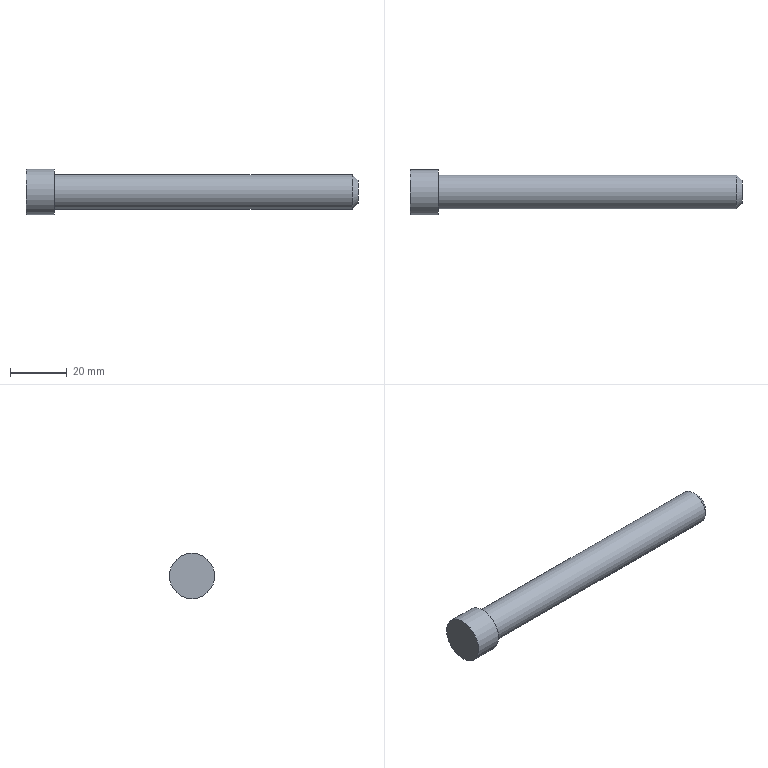Part | NX | features DATUM_CSYS 2, CHAMFER 1, SKETCH 1, SWP104 1, SYMBOLIC_THREAD 1 | 1 solid | 6 faces | box 117 x 16 x 16 mm | volume 14045 mm3 | plane 3 | cylinder 2 | cone 1 | commonest cylinder face diameters 12 x1 16 x1
STEP:
#1=CARTESIAN_POINT('',(-117.,0.,8.));
#2=VERTEX_POINT('',#1);
#3=CARTESIAN_POINT('',(-117.,0.,0.));
#4=DIRECTION('',(-1.,0.,0.));
#5=DIRECTION('',(0.,0.,1.));
#6=AXIS2_PLACEMENT_3D('',#3,#4,#5);
#7=CIRCLE('',#6,8.);
#8=EDGE_CURVE('',#2,#2,#7,.T.);
#9=ORIENTED_EDGE('',*,*,#8,.T.);
#10=EDGE_LOOP('',(#9));
#11=FACE_BOUND('',#10,.T.);
#12=CARTESIAN_POINT('',(-117.,0.,0.));
#13=DIRECTION('',(-1.,0.,0.));
#14=DIRECTION('',(0.,0.,1.));
#15=AXIS2_PLACEMENT_3D('',#12,#13,#14);
#16=PLANE('',#15);
#17=ADVANCED_FACE('',(#11),#16,.T.);
#18=CARTESIAN_POINT('',(-107.,0.,8.));
#19=VERTEX_POINT('',#18);
#20=CARTESIAN_POINT('',(-107.,0.,0.));
#21=DIRECTION('',(-1.,0.,0.));
#22=DIRECTION('',(0.,0.,1.));
#23=AXIS2_PLACEMENT_3D('',#20,#21,#22);
#24=CIRCLE('',#23,8.);
#25=EDGE_CURVE('',#19,#19,#24,.T.);
#26=ORIENTED_EDGE('',*,*,#25,.T.);
#27=EDGE_LOOP('',(#26));
#28=FACE_BOUND('',#27,.T.);
#29=ORIENTED_EDGE('',*,*,#8,.F.);
#30=EDGE_LOOP('',(#29));
#31=FACE_BOUND('',#30,.T.);
#32=CARTESIAN_POINT('',(0.,0.,0.));
#33=DIRECTION('',(-1.,0.,0.));
#34=DIRECTION('',(0.,0.,1.));
#35=AXIS2_PLACEMENT_3D('',#32,#33,#34);
#36=CYLINDRICAL_SURFACE('',#35,8.);
#37=ADVANCED_FACE('',(#28,#31),#36,.T.);
#38=CARTESIAN_POINT('',(-107.,0.,6.));
#39=VERTEX_POINT('',#38);
#40=CARTESIAN_POINT('',(-107.,0.,0.));
#41=DIRECTION('',(-1.,0.,0.));
#42=DIRECTION('',(0.,0.,1.));
#43=AXIS2_PLACEMENT_3D('',#40,#41,#42);
#44=CIRCLE('',#43,6.);
#45=EDGE_CURVE('',#39,#39,#44,.T.);
#46=ORIENTED_EDGE('',*,*,#45,.T.);
#47=EDGE_LOOP('',(#46));
#48=FACE_BOUND('',#47,.T.);
#49=ORIENTED_EDGE('',*,*,#25,.F.);
#50=EDGE_LOOP('',(#49));
#51=FACE_BOUND('',#50,.T.);
#52=CARTESIAN_POINT('',(-107.,-8.,0.));
#53=DIRECTION('',(1.,0.,0.));
#54=DIRECTION('',(0.,0.,-1.));
#55=AXIS2_PLACEMENT_3D('',#52,#53,#54);
#56=PLANE('',#55);
#57=ADVANCED_FACE('',(#48,#51),#56,.T.);
#58=CARTESIAN_POINT('',(-2.,0.,-6.));
#59=VERTEX_POINT('',#58);
#60=CARTESIAN_POINT('',(-2.,0.,0.));
#61=DIRECTION('',(1.,0.,0.));
#62=DIRECTION('',(0.,0.,-1.));
#63=AXIS2_PLACEMENT_3D('',#60,#61,#62);
#64=CIRCLE('',#63,6.);
#65=EDGE_CURVE('',#59,#59,#64,.F.);
#66=ORIENTED_EDGE('',*,*,#65,.T.);
#67=EDGE_LOOP('',(#66));
#68=FACE_BOUND('',#67,.T.);
#69=ORIENTED_EDGE('',*,*,#45,.F.);
#70=EDGE_LOOP('',(#69));
#71=FACE_BOUND('',#70,.T.);
#72=CARTESIAN_POINT('',(0.,0.,0.));
#73=DIRECTION('',(-1.,0.,0.));
#74=DIRECTION('',(0.,0.,1.));
#75=AXIS2_PLACEMENT_3D('',#72,#73,#74);
#76=CYLINDRICAL_SURFACE('',#75,6.);
#77=ADVANCED_FACE('',(#68,#71),#76,.T.);
#78=CARTESIAN_POINT('',(0.,0.,-4.));
#79=VERTEX_POINT('',#78);
#80=CARTESIAN_POINT('',(0.,0.,0.));
#81=DIRECTION('',(1.,0.,0.));
#82=DIRECTION('',(0.,0.,-1.));
#83=AXIS2_PLACEMENT_3D('',#80,#81,#82);
#84=CIRCLE('',#83,4.);
#85=EDGE_CURVE('',#79,#79,#84,.T.);
#86=ORIENTED_EDGE('',*,*,#85,.T.);
#87=EDGE_LOOP('',(#86));
#88=FACE_BOUND('',#87,.T.);
#89=CARTESIAN_POINT('',(0.,-6.,0.));
#90=DIRECTION('',(1.,0.,0.));
#91=DIRECTION('',(0.,0.,-1.));
#92=AXIS2_PLACEMENT_3D('',#89,#90,#91);
#93=PLANE('',#92);
#94=ADVANCED_FACE('',(#88),#93,.T.);
#95=ORIENTED_EDGE('',*,*,#85,.F.);
#96=EDGE_LOOP('',(#95));
#97=FACE_BOUND('',#96,.T.);
#98=ORIENTED_EDGE('',*,*,#65,.F.);
#99=EDGE_LOOP('',(#98));
#100=FACE_BOUND('',#99,.T.);
#101=CARTESIAN_POINT('',(-2.,0.,0.));
#102=DIRECTION('',(-1.,0.,0.));
#103=DIRECTION('',(0.,0.,1.));
#104=AXIS2_PLACEMENT_3D('',#101,#102,#103);
#105=CONICAL_SURFACE('',#104,6.,0.7854);
#106=ADVANCED_FACE('',(#97,#100),#105,.T.);
#107=CLOSED_SHELL('',(#17,#37,#57,#77,#94,#106));
#108=MANIFOLD_SOLID_BREP('',#107);
#109=(LENGTH_UNIT()NAMED_UNIT(*)SI_UNIT(.MILLI.,.METRE.));
#110=UNCERTAINTY_MEASURE_WITH_UNIT(LENGTH_MEASURE(0.00001),#109,'','');
#111=(NAMED_UNIT(*)PLANE_ANGLE_UNIT()SI_UNIT($,.RADIAN.));
#112=(NAMED_UNIT(*)SI_UNIT($,.STERADIAN.)SOLID_ANGLE_UNIT());
#113=(GEOMETRIC_REPRESENTATION_CONTEXT(3)GLOBAL_UNCERTAINTY_ASSIGNED_CONTEXT((#110))GLOBAL_UNIT_ASSIGNED_CONTEXT((#109,#111,#112))REPRESENTATION_CONTEXT('',''));
#114=ADVANCED_BREP_SHAPE_REPRESENTATION('',(#108),#113);